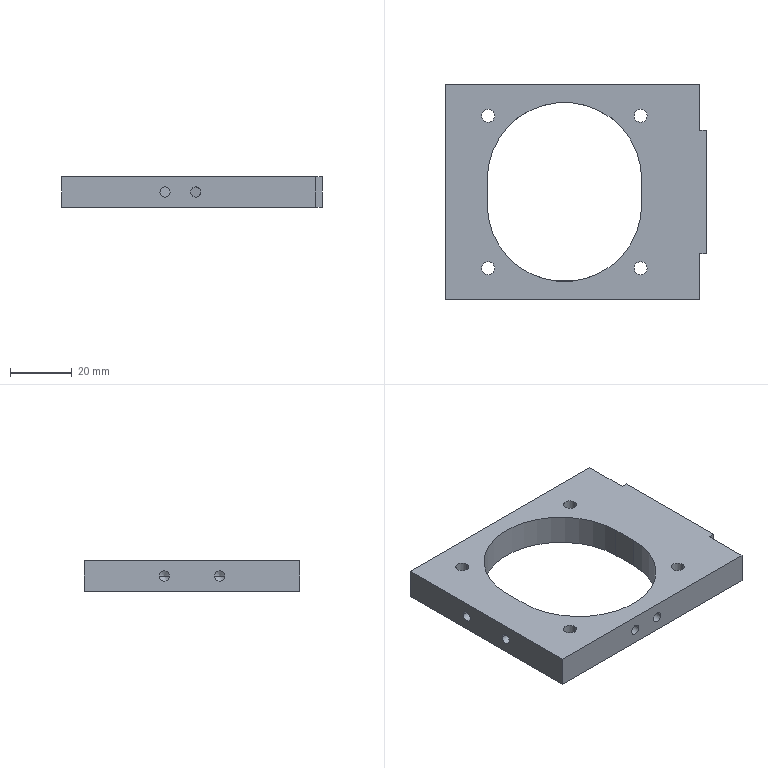Part | 1 solid | 42 faces | box 84.5 x 70 x 10 mm | volume 33501 mm3 | cylinder 22 | plane 12 | cone 8 | commonest cylinder face diameters 4.2 x12 3.3 x8 50.2 x2
STEP:
#1=CARTESIAN_POINT('',(-32.25,-7.35,-5.));
#2=VERTEX_POINT('',#1);
#3=CARTESIAN_POINT('',(-32.25,-10.65,-5.));
#4=VERTEX_POINT('',#3);
#5=CARTESIAN_POINT('',(-32.25,-9.,-5.));
#6=DIRECTION('',(-1.,0.,0.));
#7=DIRECTION('',(0.,-1.,0.));
#8=AXIS2_PLACEMENT_3D('',#5,#6,#7);
#9=CIRCLE('',#8,1.65);
#10=EDGE_CURVE('',#2,#4,#9,.T.);
#11=ORIENTED_EDGE('',*,*,#10,.F.);
#12=CARTESIAN_POINT('',(-42.25,-7.35,-5.));
#13=VERTEX_POINT('',#12);
#14=CARTESIAN_POINT('',(-42.25,-7.35,-5.));
#15=DIRECTION('',(-1.,0.,0.));
#16=VECTOR('',#15,1000.);
#17=LINE('',#14,#16);
#18=EDGE_CURVE('',#2,#13,#17,.T.);
#19=ORIENTED_EDGE('',*,*,#18,.T.);
#20=CARTESIAN_POINT('',(-42.25,-10.65,-5.));
#21=VERTEX_POINT('',#20);
#22=CARTESIAN_POINT('',(-42.25,-9.,-5.));
#23=DIRECTION('',(-1.,0.,0.));
#24=DIRECTION('',(0.,-1.,0.));
#25=AXIS2_PLACEMENT_3D('',#22,#23,#24);
#26=CIRCLE('',#25,1.65);
#27=EDGE_CURVE('',#13,#21,#26,.T.);
#28=ORIENTED_EDGE('',*,*,#27,.T.);
#29=CARTESIAN_POINT('',(-42.25,-10.65,-5.));
#30=DIRECTION('',(-1.,0.,0.));
#31=VECTOR('',#30,1000.);
#32=LINE('',#29,#31);
#33=EDGE_CURVE('',#4,#21,#32,.T.);
#34=ORIENTED_EDGE('',*,*,#33,.F.);
#35=EDGE_LOOP('',(#11,#19,#28,#34));
#36=FACE_BOUND('',#35,.T.);
#37=CARTESIAN_POINT('',(-42.25,-9.,-5.));
#38=DIRECTION('',(-1.,0.,0.));
#39=DIRECTION('',(0.,1.,0.));
#40=AXIS2_PLACEMENT_3D('',#37,#38,#39);
#41=CYLINDRICAL_SURFACE('',#40,1.65);
#42=ADVANCED_FACE('',(#36),#41,.F.);
#43=CARTESIAN_POINT('',(-31.259,-9.,-5.));
#44=VERTEX_POINT('',#43);
#45=CARTESIAN_POINT('',(-32.25,-10.65,-5.));
#46=DIRECTION('',(-0.515,-0.8572,0.));
#47=VECTOR('',#46,1000.);
#48=LINE('',#45,#47);
#49=EDGE_CURVE('',#44,#4,#48,.T.);
#50=ORIENTED_EDGE('',*,*,#49,.F.);
#51=CARTESIAN_POINT('',(-32.25,-7.35,-5.));
#52=DIRECTION('',(-0.515,0.8572,0.));
#53=VECTOR('',#52,1000.);
#54=LINE('',#51,#53);
#55=EDGE_CURVE('',#44,#2,#54,.T.);
#56=ORIENTED_EDGE('',*,*,#55,.T.);
#57=ORIENTED_EDGE('',*,*,#10,.T.);
#58=EDGE_LOOP('',(#50,#56,#57));
#59=FACE_BOUND('',#58,.T.);
#60=CARTESIAN_POINT('',(-32.25,-9.,-5.));
#61=DIRECTION('',(-1.,0.,0.));
#62=DIRECTION('',(0.,1.,0.));
#63=AXIS2_PLACEMENT_3D('',#60,#61,#62);
#64=CONICAL_SURFACE('',#63,1.65,1.03);
#65=ADVANCED_FACE('',(#59),#64,.F.);
#66=CARTESIAN_POINT('',(-32.25,10.65,-5.));
#67=VERTEX_POINT('',#66);
#68=CARTESIAN_POINT('',(-32.25,7.35,-5.));
#69=VERTEX_POINT('',#68);
#70=CARTESIAN_POINT('',(-32.25,9.,-5.));
#71=DIRECTION('',(-1.,0.,0.));
#72=DIRECTION('',(0.,-1.,0.));
#73=AXIS2_PLACEMENT_3D('',#70,#71,#72);
#74=CIRCLE('',#73,1.65);
#75=EDGE_CURVE('',#67,#69,#74,.T.);
#76=ORIENTED_EDGE('',*,*,#75,.F.);
#77=CARTESIAN_POINT('',(-42.25,10.65,-5.));
#78=VERTEX_POINT('',#77);
#79=CARTESIAN_POINT('',(-42.25,10.65,-5.));
#80=DIRECTION('',(-1.,0.,0.));
#81=VECTOR('',#80,1000.);
#82=LINE('',#79,#81);
#83=EDGE_CURVE('',#67,#78,#82,.T.);
#84=ORIENTED_EDGE('',*,*,#83,.T.);
#85=CARTESIAN_POINT('',(-42.25,7.35,-5.));
#86=VERTEX_POINT('',#85);
#87=CARTESIAN_POINT('',(-42.25,9.,-5.));
#88=DIRECTION('',(-1.,0.,0.));
#89=DIRECTION('',(0.,-1.,0.));
#90=AXIS2_PLACEMENT_3D('',#87,#88,#89);
#91=CIRCLE('',#90,1.65);
#92=EDGE_CURVE('',#78,#86,#91,.T.);
#93=ORIENTED_EDGE('',*,*,#92,.T.);
#94=CARTESIAN_POINT('',(-42.25,7.35,-5.));
#95=DIRECTION('',(-1.,0.,0.));
#96=VECTOR('',#95,1000.);
#97=LINE('',#94,#96);
#98=EDGE_CURVE('',#69,#86,#97,.T.);
#99=ORIENTED_EDGE('',*,*,#98,.F.);
#100=EDGE_LOOP('',(#76,#84,#93,#99));
#101=FACE_BOUND('',#100,.T.);
#102=CARTESIAN_POINT('',(-42.25,9.,-5.));
#103=DIRECTION('',(-1.,0.,0.));
#104=DIRECTION('',(0.,1.,0.));
#105=AXIS2_PLACEMENT_3D('',#102,#103,#104);
#106=CYLINDRICAL_SURFACE('',#105,1.65);
#107=ADVANCED_FACE('',(#101),#106,.F.);
#108=CARTESIAN_POINT('',(-31.259,9.,-5.));
#109=VERTEX_POINT('',#108);
#110=CARTESIAN_POINT('',(-32.25,7.35,-5.));
#111=DIRECTION('',(-0.515,-0.8572,0.));
#112=VECTOR('',#111,1000.);
#113=LINE('',#110,#112);
#114=EDGE_CURVE('',#109,#69,#113,.T.);
#115=ORIENTED_EDGE('',*,*,#114,.F.);
#116=CARTESIAN_POINT('',(-32.25,10.65,-5.));
#117=DIRECTION('',(-0.515,0.8572,0.));
#118=VECTOR('',#117,1000.);
#119=LINE('',#116,#118);
#120=EDGE_CURVE('',#109,#67,#119,.T.);
#121=ORIENTED_EDGE('',*,*,#120,.T.);
#122=ORIENTED_EDGE('',*,*,#75,.T.);
#123=EDGE_LOOP('',(#115,#121,#122));
#124=FACE_BOUND('',#123,.T.);
#125=CARTESIAN_POINT('',(-32.25,9.,-5.));
#126=DIRECTION('',(-1.,0.,0.));
#127=DIRECTION('',(0.,1.,0.));
#128=AXIS2_PLACEMENT_3D('',#125,#126,#127);
#129=CONICAL_SURFACE('',#128,1.65,1.03);
#130=ADVANCED_FACE('',(#124),#129,.F.);
#131=CARTESIAN_POINT('',(-10.4,-28.203,-5.));
#132=VERTEX_POINT('',#131);
#133=CARTESIAN_POINT('',(-7.1,-28.875,-5.));
#134=VERTEX_POINT('',#133);
#135=CARTESIAN_POINT('',(-10.4,-28.203,-5.));
#136=CARTESIAN_POINT('',(-10.4,-28.203,-5.441));
#137=CARTESIAN_POINT('',(-10.032,-28.308,-6.297));
#138=CARTESIAN_POINT('',(-8.762,-28.609,-6.824));
#139=CARTESIAN_POINT('',(-7.469,-28.83,-6.305));
#140=CARTESIAN_POINT('',(-7.1,-28.875,-5.441));
#141=CARTESIAN_POINT('',(-7.1,-28.875,-5.));
#142=B_SPLINE_CURVE_WITH_KNOTS('',3,(#135,#136,#137,#138,#139,#140,#141),.UNSPECIFIED.,.F.,.F.,(4,1,1,1,4),(0.,0.001303,0.002606,0.00391,0.005213),.UNSPECIFIED.);
#143=EDGE_CURVE('',#132,#134,#142,.T.);
#144=ORIENTED_EDGE('',*,*,#143,.F.);
#145=CARTESIAN_POINT('',(-10.4,-35.,-5.));
#146=VERTEX_POINT('',#145);
#147=CARTESIAN_POINT('',(-10.4,-35.,-5.));
#148=DIRECTION('',(0.,-1.,0.));
#149=VECTOR('',#148,1000.);
#150=LINE('',#147,#149);
#151=EDGE_CURVE('',#132,#146,#150,.T.);
#152=ORIENTED_EDGE('',*,*,#151,.T.);
#153=CARTESIAN_POINT('',(-7.1,-35.,-5.));
#154=VERTEX_POINT('',#153);
#155=CARTESIAN_POINT('',(-8.75,-35.,-5.));
#156=DIRECTION('',(0.,-1.,0.));
#157=DIRECTION('',(1.,0.,0.));
#158=AXIS2_PLACEMENT_3D('',#155,#156,#157);
#159=CIRCLE('',#158,1.65);
#160=EDGE_CURVE('',#146,#154,#159,.T.);
#161=ORIENTED_EDGE('',*,*,#160,.T.);
#162=CARTESIAN_POINT('',(-7.1,-35.,-5.));
#163=DIRECTION('',(0.,-1.,0.));
#164=VECTOR('',#163,1000.);
#165=LINE('',#162,#164);
#166=EDGE_CURVE('',#134,#154,#165,.T.);
#167=ORIENTED_EDGE('',*,*,#166,.F.);
#168=EDGE_LOOP('',(#144,#152,#161,#167));
#169=FACE_BOUND('',#168,.T.);
#170=CARTESIAN_POINT('',(-8.75,-35.,-5.));
#171=DIRECTION('',(0.,-1.,0.));
#172=DIRECTION('',(-1.,0.,0.));
#173=AXIS2_PLACEMENT_3D('',#170,#171,#172);
#174=CYLINDRICAL_SURFACE('',#173,1.65);
#175=ADVANCED_FACE('',(#169),#174,.F.);
#176=CARTESIAN_POINT('',(-0.4,-28.875,-5.));
#177=VERTEX_POINT('',#176);
#178=CARTESIAN_POINT('',(2.9,-28.203,-5.));
#179=VERTEX_POINT('',#178);
#180=CARTESIAN_POINT('',(-0.4,-28.875,-5.));
#181=CARTESIAN_POINT('',(-0.4,-28.875,-5.441));
#182=CARTESIAN_POINT('',(-0.03213,-28.83,-6.304));
#183=CARTESIAN_POINT('',(1.261,-28.609,-6.825));
#184=CARTESIAN_POINT('',(2.532,-28.308,-6.298));
#185=CARTESIAN_POINT('',(2.9,-28.203,-5.441));
#186=CARTESIAN_POINT('',(2.9,-28.203,-5.));
#187=B_SPLINE_CURVE_WITH_KNOTS('',3,(#180,#181,#182,#183,#184,#185,#186),.UNSPECIFIED.,.F.,.F.,(4,1,1,1,4),(0.,0.001303,0.002607,0.00391,0.005213),.UNSPECIFIED.);
#188=EDGE_CURVE('',#177,#179,#187,.T.);
#189=ORIENTED_EDGE('',*,*,#188,.F.);
#190=CARTESIAN_POINT('',(-0.4,-35.,-5.));
#191=VERTEX_POINT('',#190);
#192=CARTESIAN_POINT('',(-0.4,-35.,-5.));
#193=DIRECTION('',(0.,-1.,0.));
#194=VECTOR('',#193,1000.);
#195=LINE('',#192,#194);
#196=EDGE_CURVE('',#177,#191,#195,.T.);
#197=ORIENTED_EDGE('',*,*,#196,.T.);
#198=CARTESIAN_POINT('',(2.9,-35.,-5.));
#199=VERTEX_POINT('',#198);
#200=CARTESIAN_POINT('',(1.25,-35.,-5.));
#201=DIRECTION('',(0.,-1.,0.));
#202=DIRECTION('',(1.,0.,0.));
#203=AXIS2_PLACEMENT_3D('',#200,#201,#202);
#204=CIRCLE('',#203,1.65);
#205=EDGE_CURVE('',#191,#199,#204,.T.);
#206=ORIENTED_EDGE('',*,*,#205,.T.);
#207=CARTESIAN_POINT('',(2.9,-35.,-5.));
#208=DIRECTION('',(0.,-1.,0.));
#209=VECTOR('',#208,1000.);
#210=LINE('',#207,#209);
#211=EDGE_CURVE('',#179,#199,#210,.T.);
#212=ORIENTED_EDGE('',*,*,#211,.F.);
#213=EDGE_LOOP('',(#189,#197,#206,#212));
#214=FACE_BOUND('',#213,.T.);
#215=CARTESIAN_POINT('',(1.25,-35.,-5.));
#216=DIRECTION('',(0.,-1.,0.));
#217=DIRECTION('',(-1.,0.,0.));
#218=AXIS2_PLACEMENT_3D('',#215,#216,#217);
#219=CYLINDRICAL_SURFACE('',#218,1.65);
#220=ADVANCED_FACE('',(#214),#219,.F.);
#221=CARTESIAN_POINT('',(28.25,10.4,-5.));
#222=VERTEX_POINT('',#221);
#223=CARTESIAN_POINT('',(28.25,14.6,-5.));
#224=VERTEX_POINT('',#223);
#225=CARTESIAN_POINT('',(28.25,12.5,-5.));
#226=DIRECTION('',(1.,0.,0.));
#227=DIRECTION('',(0.,1.,0.));
#228=AXIS2_PLACEMENT_3D('',#225,#226,#227);
#229=CIRCLE('',#228,2.1);
#230=EDGE_CURVE('',#222,#224,#229,.T.);
#231=ORIENTED_EDGE('',*,*,#230,.F.);
#232=CARTESIAN_POINT('',(42.25,10.4,-5.));
#233=VERTEX_POINT('',#232);
#234=CARTESIAN_POINT('',(42.25,10.4,-5.));
#235=DIRECTION('',(1.,0.,0.));
#236=VECTOR('',#235,1000.);
#237=LINE('',#234,#236);
#238=EDGE_CURVE('',#222,#233,#237,.T.);
#239=ORIENTED_EDGE('',*,*,#238,.T.);
#240=CARTESIAN_POINT('',(42.25,14.6,-5.));
#241=VERTEX_POINT('',#240);
#242=CARTESIAN_POINT('',(42.25,12.5,-5.));
#243=DIRECTION('',(1.,0.,0.));
#244=DIRECTION('',(0.,1.,0.));
#245=AXIS2_PLACEMENT_3D('',#242,#243,#244);
#246=CIRCLE('',#245,2.1);
#247=EDGE_CURVE('',#233,#241,#246,.T.);
#248=ORIENTED_EDGE('',*,*,#247,.T.);
#249=CARTESIAN_POINT('',(42.25,14.6,-5.));
#250=DIRECTION('',(1.,0.,0.));
#251=VECTOR('',#250,1000.);
#252=LINE('',#249,#251);
#253=EDGE_CURVE('',#224,#241,#252,.T.);
#254=ORIENTED_EDGE('',*,*,#253,.F.);
#255=EDGE_LOOP('',(#231,#239,#248,#254));
#256=FACE_BOUND('',#255,.T.);
#257=CARTESIAN_POINT('',(42.25,12.5,-5.));
#258=DIRECTION('',(1.,0.,0.));
#259=DIRECTION('',(0.,-1.,0.));
#260=AXIS2_PLACEMENT_3D('',#257,#258,#259);
#261=CYLINDRICAL_SURFACE('',#260,2.1);
#262=ADVANCED_FACE('',(#256),#261,.F.);
#263=CARTESIAN_POINT('',(26.988,12.5,-5.));
#264=VERTEX_POINT('',#263);
#265=CARTESIAN_POINT('',(28.25,14.6,-5.));
#266=DIRECTION('',(0.515,0.8572,0.));
#267=VECTOR('',#266,1000.);
#268=LINE('',#265,#267);
#269=EDGE_CURVE('',#264,#224,#268,.T.);
#270=ORIENTED_EDGE('',*,*,#269,.F.);
#271=CARTESIAN_POINT('',(28.25,10.4,-5.));
#272=DIRECTION('',(0.515,-0.8572,0.));
#273=VECTOR('',#272,1000.);
#274=LINE('',#271,#273);
#275=EDGE_CURVE('',#264,#222,#274,.T.);
#276=ORIENTED_EDGE('',*,*,#275,.T.);
#277=ORIENTED_EDGE('',*,*,#230,.T.);
#278=EDGE_LOOP('',(#270,#276,#277));
#279=FACE_BOUND('',#278,.T.);
#280=CARTESIAN_POINT('',(28.25,12.5,-5.));
#281=DIRECTION('',(1.,0.,0.));
#282=DIRECTION('',(0.,-1.,0.));
#283=AXIS2_PLACEMENT_3D('',#280,#281,#282);
#284=CONICAL_SURFACE('',#283,2.1,1.03);
#285=ADVANCED_FACE('',(#279),#284,.F.);
#286=CARTESIAN_POINT('',(28.25,-14.6,-5.));
#287=VERTEX_POINT('',#286);
#288=CARTESIAN_POINT('',(28.25,-10.4,-5.));
#289=VERTEX_POINT('',#288);
#290=CARTESIAN_POINT('',(28.25,-12.5,-5.));
#291=DIRECTION('',(1.,0.,0.));
#292=DIRECTION('',(0.,1.,0.));
#293=AXIS2_PLACEMENT_3D('',#290,#291,#292);
#294=CIRCLE('',#293,2.1);
#295=EDGE_CURVE('',#287,#289,#294,.T.);
#296=ORIENTED_EDGE('',*,*,#295,.F.);
#297=CARTESIAN_POINT('',(42.25,-14.6,-5.));
#298=VERTEX_POINT('',#297);
#299=CARTESIAN_POINT('',(42.25,-14.6,-5.));
#300=DIRECTION('',(1.,0.,0.));
#301=VECTOR('',#300,1000.);
#302=LINE('',#299,#301);
#303=EDGE_CURVE('',#287,#298,#302,.T.);
#304=ORIENTED_EDGE('',*,*,#303,.T.);
#305=CARTESIAN_POINT('',(42.25,-10.4,-5.));
#306=VERTEX_POINT('',#305);
#307=CARTESIAN_POINT('',(42.25,-12.5,-5.));
#308=DIRECTION('',(1.,0.,0.));
#309=DIRECTION('',(0.,1.,0.));
#310=AXIS2_PLACEMENT_3D('',#307,#308,#309);
#311=CIRCLE('',#310,2.1);
#312=EDGE_CURVE('',#298,#306,#311,.T.);
#313=ORIENTED_EDGE('',*,*,#312,.T.);
#314=CARTESIAN_POINT('',(42.25,-10.4,-5.));
#315=DIRECTION('',(1.,0.,0.));
#316=VECTOR('',#315,1000.);
#317=LINE('',#314,#316);
#318=EDGE_CURVE('',#289,#306,#317,.T.);
#319=ORIENTED_EDGE('',*,*,#318,.F.);
#320=EDGE_LOOP('',(#296,#304,#313,#319));
#321=FACE_BOUND('',#320,.T.);
#322=CARTESIAN_POINT('',(42.25,-12.5,-5.));
#323=DIRECTION('',(1.,0.,0.));
#324=DIRECTION('',(0.,-1.,0.));
#325=AXIS2_PLACEMENT_3D('',#322,#323,#324);
#326=CYLINDRICAL_SURFACE('',#325,2.1);
#327=ADVANCED_FACE('',(#321),#326,.F.);
#328=CARTESIAN_POINT('',(26.988,-12.5,-5.));
#329=VERTEX_POINT('',#328);
#330=CARTESIAN_POINT('',(28.25,-10.4,-5.));
#331=DIRECTION('',(0.515,0.8572,0.));
#332=VECTOR('',#331,1000.);
#333=LINE('',#330,#332);
#334=EDGE_CURVE('',#329,#289,#333,.T.);
#335=ORIENTED_EDGE('',*,*,#334,.F.);
#336=CARTESIAN_POINT('',(28.25,-14.6,-5.));
#337=DIRECTION('',(0.515,-0.8572,0.));
#338=VECTOR('',#337,1000.);
#339=LINE('',#336,#338);
#340=EDGE_CURVE('',#329,#287,#339,.T.);
#341=ORIENTED_EDGE('',*,*,#340,.T.);
#342=ORIENTED_EDGE('',*,*,#295,.T.);
#343=EDGE_LOOP('',(#335,#341,#342));
#344=FACE_BOUND('',#343,.T.);
#345=CARTESIAN_POINT('',(28.25,-12.5,-5.));
#346=DIRECTION('',(1.,0.,0.));
#347=DIRECTION('',(0.,-1.,0.));
#348=AXIS2_PLACEMENT_3D('',#345,#346,#347);
#349=CONICAL_SURFACE('',#348,2.1,1.03);
#350=ADVANCED_FACE('',(#344),#349,.F.);
#351=CARTESIAN_POINT('',(-26.4,24.75,0.));
#352=VERTEX_POINT('',#351);
#353=CARTESIAN_POINT('',(-30.6,24.75,0.));
#354=VERTEX_POINT('',#353);
#355=CARTESIAN_POINT('',(-28.5,24.75,0.));
#356=DIRECTION('',(0.,0.,-1.));
#357=DIRECTION('',(-1.,0.,0.));
#358=AXIS2_PLACEMENT_3D('',#355,#356,#357);
#359=CIRCLE('',#358,2.1);
#360=EDGE_CURVE('',#352,#354,#359,.T.);
#361=ORIENTED_EDGE('',*,*,#360,.F.);
#362=CARTESIAN_POINT('',(-26.4,24.75,-10.));
#363=VERTEX_POINT('',#362);
#364=CARTESIAN_POINT('',(-26.4,24.75,-10.));
#365=DIRECTION('',(0.,0.,-1.));
#366=VECTOR('',#365,1000.);
#367=LINE('',#364,#366);
#368=EDGE_CURVE('',#352,#363,#367,.T.);
#369=ORIENTED_EDGE('',*,*,#368,.T.);
#370=CARTESIAN_POINT('',(-30.6,24.75,-10.));
#371=VERTEX_POINT('',#370);
#372=CARTESIAN_POINT('',(-28.5,24.75,-10.));
#373=DIRECTION('',(0.,0.,-1.));
#374=DIRECTION('',(-1.,0.,0.));
#375=AXIS2_PLACEMENT_3D('',#372,#373,#374);
#376=CIRCLE('',#375,2.1);
#377=EDGE_CURVE('',#363,#371,#376,.T.);
#378=ORIENTED_EDGE('',*,*,#377,.T.);
#379=CARTESIAN_POINT('',(-30.6,24.75,-10.));
#380=DIRECTION('',(0.,0.,-1.));
#381=VECTOR('',#380,1000.);
#382=LINE('',#379,#381);
#383=EDGE_CURVE('',#354,#371,#382,.T.);
#384=ORIENTED_EDGE('',*,*,#383,.F.);
#385=EDGE_LOOP('',(#361,#369,#378,#384));
#386=FACE_BOUND('',#385,.T.);
#387=CARTESIAN_POINT('',(-28.5,24.75,-10.));
#388=DIRECTION('',(0.,0.,-1.));
#389=DIRECTION('',(1.,0.,0.));
#390=AXIS2_PLACEMENT_3D('',#387,#388,#389);
#391=CYLINDRICAL_SURFACE('',#390,2.1);
#392=ADVANCED_FACE('',(#386),#391,.F.);
#393=CARTESIAN_POINT('',(-26.4,-24.75,0.));
#394=VERTEX_POINT('',#393);
#395=CARTESIAN_POINT('',(-30.6,-24.75,0.));
#396=VERTEX_POINT('',#395);
#397=CARTESIAN_POINT('',(-28.5,-24.75,0.));
#398=DIRECTION('',(0.,0.,-1.));
#399=DIRECTION('',(-1.,0.,0.));
#400=AXIS2_PLACEMENT_3D('',#397,#398,#399);
#401=CIRCLE('',#400,2.1);
#402=EDGE_CURVE('',#394,#396,#401,.T.);
#403=ORIENTED_EDGE('',*,*,#402,.F.);
#404=CARTESIAN_POINT('',(-26.4,-24.75,-10.));
#405=VERTEX_POINT('',#404);
#406=CARTESIAN_POINT('',(-26.4,-24.75,-10.));
#407=DIRECTION('',(0.,0.,-1.));
#408=VECTOR('',#407,1000.);
#409=LINE('',#406,#408);
#410=EDGE_CURVE('',#394,#405,#409,.T.);
#411=ORIENTED_EDGE('',*,*,#410,.T.);
#412=CARTESIAN_POINT('',(-30.6,-24.75,-10.));
#413=VERTEX_POINT('',#412);
#414=CARTESIAN_POINT('',(-28.5,-24.75,-10.));
#415=DIRECTION('',(0.,0.,-1.));
#416=DIRECTION('',(-1.,0.,0.));
#417=AXIS2_PLACEMENT_3D('',#414,#415,#416);
#418=CIRCLE('',#417,2.1);
#419=EDGE_CURVE('',#405,#413,#418,.T.);
#420=ORIENTED_EDGE('',*,*,#419,.T.);
#421=CARTESIAN_POINT('',(-30.6,-24.75,-10.));
#422=DIRECTION('',(0.,0.,-1.));
#423=VECTOR('',#422,1000.);
#424=LINE('',#421,#423);
#425=EDGE_CURVE('',#396,#413,#424,.T.);
#426=ORIENTED_EDGE('',*,*,#425,.F.);
#427=EDGE_LOOP('',(#403,#411,#420,#426));
#428=FACE_BOUND('',#427,.T.);
#429=CARTESIAN_POINT('',(-28.5,-24.75,-10.));
#430=DIRECTION('',(0.,0.,-1.));
#431=DIRECTION('',(1.,0.,0.));
#432=AXIS2_PLACEMENT_3D('',#429,#430,#431);
#433=CYLINDRICAL_SURFACE('',#432,2.1);
#434=ADVANCED_FACE('',(#428),#433,.F.);
#435=CARTESIAN_POINT('',(23.1,24.75,0.));
#436=VERTEX_POINT('',#435);
#437=CARTESIAN_POINT('',(18.9,24.75,0.));
#438=VERTEX_POINT('',#437);
#439=CARTESIAN_POINT('',(21.,24.75,0.));
#440=DIRECTION('',(0.,0.,-1.));
#441=DIRECTION('',(-1.,0.,0.));
#442=AXIS2_PLACEMENT_3D('',#439,#440,#441);
#443=CIRCLE('',#442,2.1);
#444=EDGE_CURVE('',#436,#438,#443,.T.);
#445=ORIENTED_EDGE('',*,*,#444,.F.);
#446=CARTESIAN_POINT('',(23.1,24.75,-10.));
#447=VERTEX_POINT('',#446);
#448=CARTESIAN_POINT('',(23.1,24.75,-10.));
#449=DIRECTION('',(0.,0.,-1.));
#450=VECTOR('',#449,1000.);
#451=LINE('',#448,#450);
#452=EDGE_CURVE('',#436,#447,#451,.T.);
#453=ORIENTED_EDGE('',*,*,#452,.T.);
#454=CARTESIAN_POINT('',(18.9,24.75,-10.));
#455=VERTEX_POINT('',#454);
#456=CARTESIAN_POINT('',(21.,24.75,-10.));
#457=DIRECTION('',(0.,0.,-1.));
#458=DIRECTION('',(-1.,0.,0.));
#459=AXIS2_PLACEMENT_3D('',#456,#457,#458);
#460=CIRCLE('',#459,2.1);
#461=EDGE_CURVE('',#447,#455,#460,.T.);
#462=ORIENTED_EDGE('',*,*,#461,.T.);
#463=CARTESIAN_POINT('',(18.9,24.75,-10.));
#464=DIRECTION('',(0.,0.,-1.));
#465=VECTOR('',#464,1000.);
#466=LINE('',#463,#465);
#467=EDGE_CURVE('',#438,#455,#466,.T.);
#468=ORIENTED_EDGE('',*,*,#467,.F.);
#469=EDGE_LOOP('',(#445,#453,#462,#468));
#470=FACE_BOUND('',#469,.T.);
#471=CARTESIAN_POINT('',(21.,24.75,-10.));
#472=DIRECTION('',(0.,0.,-1.));
#473=DIRECTION('',(1.,0.,0.));
#474=AXIS2_PLACEMENT_3D('',#471,#472,#473);
#475=CYLINDRICAL_SURFACE('',#474,2.1);
#476=ADVANCED_FACE('',(#470),#475,.F.);
#477=CARTESIAN_POINT('',(23.1,-24.75,0.));
#478=VERTEX_POINT('',#477);
#479=CARTESIAN_POINT('',(18.9,-24.75,0.));
#480=VERTEX_POINT('',#479);
#481=CARTESIAN_POINT('',(21.,-24.75,0.));
#482=DIRECTION('',(0.,0.,-1.));
#483=DIRECTION('',(-1.,0.,0.));
#484=AXIS2_PLACEMENT_3D('',#481,#482,#483);
#485=CIRCLE('',#484,2.1);
#486=EDGE_CURVE('',#478,#480,#485,.T.);
#487=ORIENTED_EDGE('',*,*,#486,.F.);
#488=CARTESIAN_POINT('',(23.1,-24.75,-10.));
#489=VERTEX_POINT('',#488);
#490=CARTESIAN_POINT('',(23.1,-24.75,-10.));
#491=DIRECTION('',(0.,0.,-1.));
#492=VECTOR('',#491,1000.);
#493=LINE('',#490,#492);
#494=EDGE_CURVE('',#478,#489,#493,.T.);
#495=ORIENTED_EDGE('',*,*,#494,.T.);
#496=CARTESIAN_POINT('',(18.9,-24.75,-10.));
#497=VERTEX_POINT('',#496);
#498=CARTESIAN_POINT('',(21.,-24.75,-10.));
#499=DIRECTION('',(0.,0.,-1.));
#500=DIRECTION('',(-1.,0.,0.));
#501=AXIS2_PLACEMENT_3D('',#498,#499,#500);
#502=CIRCLE('',#501,2.1);
#503=EDGE_CURVE('',#489,#497,#502,.T.);
#504=ORIENTED_EDGE('',*,*,#503,.T.);
#505=CARTESIAN_POINT('',(18.9,-24.75,-10.));
#506=DIRECTION('',(0.,0.,-1.));
#507=VECTOR('',#506,1000.);
#508=LINE('',#505,#507);
#509=EDGE_CURVE('',#480,#497,#508,.T.);
#510=ORIENTED_EDGE('',*,*,#509,.F.);
#511=EDGE_LOOP('',(#487,#495,#504,#510));
#512=FACE_BOUND('',#511,.T.);
#513=CARTESIAN_POINT('',(21.,-24.75,-10.));
#514=DIRECTION('',(0.,0.,-1.));
#515=DIRECTION('',(1.,0.,0.));
#516=AXIS2_PLACEMENT_3D('',#513,#514,#515);
#517=CYLINDRICAL_SURFACE('',#516,2.1);
#518=ADVANCED_FACE('',(#512),#517,.F.);
#519=CARTESIAN_POINT('',(40.25,35.,0.));
#520=VERTEX_POINT('',#519);
#521=CARTESIAN_POINT('',(-42.25,35.,0.));
#522=VERTEX_POINT('',#521);
#523=CARTESIAN_POINT('',(42.25,35.,0.));
#524=DIRECTION('',(-1.,0.,0.));
#525=VECTOR('',#524,1000.);
#526=LINE('',#523,#525);
#527=EDGE_CURVE('',#520,#522,#526,.T.);
#528=ORIENTED_EDGE('',*,*,#527,.F.);
#529=CARTESIAN_POINT('',(40.25,35.,-10.));
#530=VERTEX_POINT('',#529);
#531=CARTESIAN_POINT('',(40.25,35.,0.));
#532=DIRECTION('',(0.,0.,-1.));
#533=VECTOR('',#532,1000.);
#534=LINE('',#531,#533);
#535=EDGE_CURVE('',#520,#530,#534,.T.);
#536=ORIENTED_EDGE('',*,*,#535,.T.);
#537=CARTESIAN_POINT('',(-42.25,35.,-10.));
#538=VERTEX_POINT('',#537);
#539=CARTESIAN_POINT('',(42.25,35.,-10.));
#540=DIRECTION('',(-1.,0.,0.));
#541=VECTOR('',#540,1000.);
#542=LINE('',#539,#541);
#543=EDGE_CURVE('',#530,#538,#542,.T.);
#544=ORIENTED_EDGE('',*,*,#543,.T.);
#545=CARTESIAN_POINT('',(-42.25,35.,0.));
#546=DIRECTION('',(0.,0.,-1.));
#547=VECTOR('',#546,1000.);
#548=LINE('',#545,#547);
#549=EDGE_CURVE('',#522,#538,#548,.T.);
#550=ORIENTED_EDGE('',*,*,#549,.F.);
#551=EDGE_LOOP('',(#528,#536,#544,#550));
#552=FACE_BOUND('',#551,.T.);
#553=CARTESIAN_POINT('',(42.25,35.,0.));
#554=DIRECTION('',(0.,-1.,0.));
#555=DIRECTION('',(-1.,0.,0.));
#556=AXIS2_PLACEMENT_3D('',#553,#554,#555);
#557=PLANE('',#556);
#558=ADVANCED_FACE('',(#552),#557,.F.);
#559=CARTESIAN_POINT('',(-42.25,-9.,-5.));
#560=DIRECTION('',(-1.,0.,0.));
#561=DIRECTION('',(0.,-1.,0.));
#562=AXIS2_PLACEMENT_3D('',#559,#560,#561);
#563=CIRCLE('',#562,1.65);
#564=EDGE_CURVE('',#21,#13,#563,.T.);
#565=ORIENTED_EDGE('',*,*,#564,.F.);
#566=ORIENTED_EDGE('',*,*,#27,.F.);
#567=EDGE_LOOP('',(#565,#566));
#568=FACE_BOUND('',#567,.T.);
#569=CARTESIAN_POINT('',(-42.25,9.,-5.));
#570=DIRECTION('',(-1.,0.,0.));
#571=DIRECTION('',(0.,-1.,0.));
#572=AXIS2_PLACEMENT_3D('',#569,#570,#571);
#573=CIRCLE('',#572,1.65);
#574=EDGE_CURVE('',#86,#78,#573,.T.);
#575=ORIENTED_EDGE('',*,*,#574,.F.);
#576=ORIENTED_EDGE('',*,*,#92,.F.);
#577=EDGE_LOOP('',(#575,#576));
#578=FACE_BOUND('',#577,.T.);
#579=CARTESIAN_POINT('',(-42.25,-35.,-10.));
#580=VERTEX_POINT('',#579);
#581=CARTESIAN_POINT('',(-42.25,-35.,-10.));
#582=DIRECTION('',(0.,-1.,0.));
#583=VECTOR('',#582,1000.);
#584=LINE('',#581,#583);
#585=EDGE_CURVE('',#538,#580,#584,.T.);
#586=ORIENTED_EDGE('',*,*,#585,.T.);
#587=CARTESIAN_POINT('',(-42.25,-35.,0.));
#588=VERTEX_POINT('',#587);
#589=CARTESIAN_POINT('',(-42.25,-35.,0.));
#590=DIRECTION('',(0.,0.,-1.));
#591=VECTOR('',#590,1000.);
#592=LINE('',#589,#591);
#593=EDGE_CURVE('',#588,#580,#592,.T.);
#594=ORIENTED_EDGE('',*,*,#593,.F.);
#595=CARTESIAN_POINT('',(-42.25,-35.,0.));
#596=DIRECTION('',(0.,-1.,0.));
#597=VECTOR('',#596,1000.);
#598=LINE('',#595,#597);
#599=EDGE_CURVE('',#522,#588,#598,.T.);
#600=ORIENTED_EDGE('',*,*,#599,.F.);
#601=ORIENTED_EDGE('',*,*,#549,.T.);
#602=EDGE_LOOP('',(#586,#594,#600,#601));
#603=FACE_BOUND('',#602,.T.);
#604=CARTESIAN_POINT('',(-42.25,-35.,0.));
#605=DIRECTION('',(1.,0.,0.));
#606=DIRECTION('',(0.,-1.,0.));
#607=AXIS2_PLACEMENT_3D('',#604,#605,#606);
#608=PLANE('',#607);
#609=ADVANCED_FACE('',(#568,#578,#603),#608,.F.);
#610=CARTESIAN_POINT('',(-8.75,-35.,-5.));
#611=DIRECTION('',(0.,-1.,0.));
#612=DIRECTION('',(1.,0.,0.));
#613=AXIS2_PLACEMENT_3D('',#610,#611,#612);
#614=CIRCLE('',#613,1.65);
#615=EDGE_CURVE('',#154,#146,#614,.T.);
#616=ORIENTED_EDGE('',*,*,#615,.F.);
#617=ORIENTED_EDGE('',*,*,#160,.F.);
#618=EDGE_LOOP('',(#616,#617));
#619=FACE_BOUND('',#618,.T.);
#620=CARTESIAN_POINT('',(1.25,-35.,-5.));
#621=DIRECTION('',(0.,-1.,0.));
#622=DIRECTION('',(1.,0.,0.));
#623=AXIS2_PLACEMENT_3D('',#620,#621,#622);
#624=CIRCLE('',#623,1.65);
#625=EDGE_CURVE('',#199,#191,#624,.T.);
#626=ORIENTED_EDGE('',*,*,#625,.F.);
#627=ORIENTED_EDGE('',*,*,#205,.F.);
#628=EDGE_LOOP('',(#626,#627));
#629=FACE_BOUND('',#628,.T.);
#630=CARTESIAN_POINT('',(40.25,-35.,-10.));
#631=VERTEX_POINT('',#630);
#632=CARTESIAN_POINT('',(42.25,-35.,-10.));
#633=DIRECTION('',(1.,0.,0.));
#634=VECTOR('',#633,1000.);
#635=LINE('',#632,#634);
#636=EDGE_CURVE('',#580,#631,#635,.T.);
#637=ORIENTED_EDGE('',*,*,#636,.T.);
#638=CARTESIAN_POINT('',(40.25,-35.,0.));
#639=VERTEX_POINT('',#638);
#640=CARTESIAN_POINT('',(40.25,-35.,0.));
#641=DIRECTION('',(0.,0.,-1.));
#642=VECTOR('',#641,1000.);
#643=LINE('',#640,#642);
#644=EDGE_CURVE('',#639,#631,#643,.T.);
#645=ORIENTED_EDGE('',*,*,#644,.F.);
#646=CARTESIAN_POINT('',(42.25,-35.,0.));
#647=DIRECTION('',(1.,0.,0.));
#648=VECTOR('',#647,1000.);
#649=LINE('',#646,#648);
#650=EDGE_CURVE('',#588,#639,#649,.T.);
#651=ORIENTED_EDGE('',*,*,#650,.F.);
#652=ORIENTED_EDGE('',*,*,#593,.T.);
#653=EDGE_LOOP('',(#637,#645,#651,#652));
#654=FACE_BOUND('',#653,.T.);
#655=CARTESIAN_POINT('',(42.25,-35.,0.));
#656=DIRECTION('',(0.,1.,0.));
#657=DIRECTION('',(1.,0.,0.));
#658=AXIS2_PLACEMENT_3D('',#655,#656,#657);
#659=PLANE('',#658);
#660=ADVANCED_FACE('',(#619,#629,#654),#659,.F.);
#661=CARTESIAN_POINT('',(42.25,12.5,-5.));
#662=DIRECTION('',(1.,0.,0.));
#663=DIRECTION('',(0.,1.,0.));
#664=AXIS2_PLACEMENT_3D('',#661,#662,#663);
#665=CIRCLE('',#664,2.1);
#666=EDGE_CURVE('',#241,#233,#665,.T.);
#667=ORIENTED_EDGE('',*,*,#666,.F.);
#668=ORIENTED_EDGE('',*,*,#247,.F.);
#669=EDGE_LOOP('',(#667,#668));
#670=FACE_BOUND('',#669,.T.);
#671=CARTESIAN_POINT('',(42.25,-12.5,-5.));
#672=DIRECTION('',(1.,0.,0.));
#673=DIRECTION('',(0.,1.,0.));
#674=AXIS2_PLACEMENT_3D('',#671,#672,#673);
#675=CIRCLE('',#674,2.1);
#676=EDGE_CURVE('',#306,#298,#675,.T.);
#677=ORIENTED_EDGE('',*,*,#676,.F.);
#678=ORIENTED_EDGE('',*,*,#312,.F.);
#679=EDGE_LOOP('',(#677,#678));
#680=FACE_BOUND('',#679,.T.);
#681=CARTESIAN_POINT('',(42.25,-20.,0.));
#682=VERTEX_POINT('',#681);
#683=CARTESIAN_POINT('',(42.25,20.,0.));
#684=VERTEX_POINT('',#683);
#685=CARTESIAN_POINT('',(42.25,-35.,0.));
#686=DIRECTION('',(0.,1.,0.));
#687=VECTOR('',#686,1000.);
#688=LINE('',#685,#687);
#689=EDGE_CURVE('',#682,#684,#688,.T.);
#690=ORIENTED_EDGE('',*,*,#689,.F.);
#691=CARTESIAN_POINT('',(42.25,-20.,-10.));
#692=VERTEX_POINT('',#691);
#693=CARTESIAN_POINT('',(42.25,-20.,0.));
#694=DIRECTION('',(0.,0.,-1.));
#695=VECTOR('',#694,1000.);
#696=LINE('',#693,#695);
#697=EDGE_CURVE('',#682,#692,#696,.T.);
#698=ORIENTED_EDGE('',*,*,#697,.T.);
#699=CARTESIAN_POINT('',(42.25,20.,-10.));
#700=VERTEX_POINT('',#699);
#701=CARTESIAN_POINT('',(42.25,-35.,-10.));
#702=DIRECTION('',(0.,1.,0.));
#703=VECTOR('',#702,1000.);
#704=LINE('',#701,#703);
#705=EDGE_CURVE('',#692,#700,#704,.T.);
#706=ORIENTED_EDGE('',*,*,#705,.T.);
#707=CARTESIAN_POINT('',(42.25,20.,0.));
#708=DIRECTION('',(0.,0.,-1.));
#709=VECTOR('',#708,1000.);
#710=LINE('',#707,#709);
#711=EDGE_CURVE('',#684,#700,#710,.T.);
#712=ORIENTED_EDGE('',*,*,#711,.F.);
#713=EDGE_LOOP('',(#690,#698,#706,#712));
#714=FACE_BOUND('',#713,.T.);
#715=CARTESIAN_POINT('',(42.25,-35.,0.));
#716=DIRECTION('',(-1.,0.,0.));
#717=DIRECTION('',(0.,1.,0.));
#718=AXIS2_PLACEMENT_3D('',#715,#716,#717);
#719=PLANE('',#718);
#720=ADVANCED_FACE('',(#670,#680,#714),#719,.F.);
#721=CARTESIAN_POINT('',(-28.5,24.75,0.));
#722=DIRECTION('',(0.,0.,-1.));
#723=DIRECTION('',(-1.,0.,0.));
#724=AXIS2_PLACEMENT_3D('',#721,#722,#723);
#725=CIRCLE('',#724,2.1);
#726=EDGE_CURVE('',#354,#352,#725,.T.);
#727=ORIENTED_EDGE('',*,*,#726,.T.);
#728=ORIENTED_EDGE('',*,*,#360,.T.);
#729=EDGE_LOOP('',(#727,#728));
#730=FACE_BOUND('',#729,.T.);
#731=CARTESIAN_POINT('',(-28.5,-24.75,0.));
#732=DIRECTION('',(0.,0.,-1.));
#733=DIRECTION('',(-1.,0.,0.));
#734=AXIS2_PLACEMENT_3D('',#731,#732,#733);
#735=CIRCLE('',#734,2.1);
#736=EDGE_CURVE('',#396,#394,#735,.T.);
#737=ORIENTED_EDGE('',*,*,#736,.T.);
#738=ORIENTED_EDGE('',*,*,#402,.T.);
#739=EDGE_LOOP('',(#737,#738));
#740=FACE_BOUND('',#739,.T.);
#741=CARTESIAN_POINT('',(21.,24.75,0.));
#742=DIRECTION('',(0.,0.,-1.));
#743=DIRECTION('',(-1.,0.,0.));
#744=AXIS2_PLACEMENT_3D('',#741,#742,#743);
#745=CIRCLE('',#744,2.1);
#746=EDGE_CURVE('',#438,#436,#745,.T.);
#747=ORIENTED_EDGE('',*,*,#746,.T.);
#748=ORIENTED_EDGE('',*,*,#444,.T.);
#749=EDGE_LOOP('',(#747,#748));
#750=FACE_BOUND('',#749,.T.);
#751=CARTESIAN_POINT('',(21.,-24.75,0.));
#752=DIRECTION('',(0.,0.,-1.));
#753=DIRECTION('',(-1.,0.,0.));
#754=AXIS2_PLACEMENT_3D('',#751,#752,#753);
#755=CIRCLE('',#754,2.1);
#756=EDGE_CURVE('',#480,#478,#755,.T.);
#757=ORIENTED_EDGE('',*,*,#756,.T.);
#758=ORIENTED_EDGE('',*,*,#486,.T.);
#759=EDGE_LOOP('',(#757,#758));
#760=FACE_BOUND('',#759,.T.);
#761=CARTESIAN_POINT('',(21.35,-4.,0.));
#762=VERTEX_POINT('',#761);
#763=CARTESIAN_POINT('',(21.35,4.,0.));
#764=VERTEX_POINT('',#763);
#765=CARTESIAN_POINT('',(21.35,-4.,0.));
#766=DIRECTION('',(0.,1.,0.));
#767=VECTOR('',#766,1000.);
#768=LINE('',#765,#767);
#769=EDGE_CURVE('',#762,#764,#768,.T.);
#770=ORIENTED_EDGE('',*,*,#769,.F.);
#771=CARTESIAN_POINT('',(-28.85,-4.,0.));
#772=VERTEX_POINT('',#771);
#773=CARTESIAN_POINT('',(-3.75,-4.,0.));
#774=DIRECTION('',(0.,0.,1.));
#775=DIRECTION('',(1.,0.,0.));
#776=AXIS2_PLACEMENT_3D('',#773,#774,#775);
#777=CIRCLE('',#776,25.1);
#778=EDGE_CURVE('',#772,#762,#777,.T.);
#779=ORIENTED_EDGE('',*,*,#778,.F.);
#780=CARTESIAN_POINT('',(-28.85,4.,0.));
#781=VERTEX_POINT('',#780);
#782=CARTESIAN_POINT('',(-28.85,-4.,0.));
#783=DIRECTION('',(0.,-1.,0.));
#784=VECTOR('',#783,1000.);
#785=LINE('',#782,#784);
#786=EDGE_CURVE('',#781,#772,#785,.T.);
#787=ORIENTED_EDGE('',*,*,#786,.F.);
#788=CARTESIAN_POINT('',(-3.75,4.,0.));
#789=DIRECTION('',(0.,0.,1.));
#790=DIRECTION('',(1.,0.,0.));
#791=AXIS2_PLACEMENT_3D('',#788,#789,#790);
#792=CIRCLE('',#791,25.1);
#793=EDGE_CURVE('',#764,#781,#792,.T.);
#794=ORIENTED_EDGE('',*,*,#793,.F.);
#795=EDGE_LOOP('',(#770,#779,#787,#794));
#796=FACE_BOUND('',#795,.T.);
#797=CARTESIAN_POINT('',(40.25,-20.,0.));
#798=VERTEX_POINT('',#797);
#799=CARTESIAN_POINT('',(40.25,-35.,0.));
#800=DIRECTION('',(0.,1.,0.));
#801=VECTOR('',#800,1000.);
#802=LINE('',#799,#801);
#803=EDGE_CURVE('',#639,#798,#802,.T.);
#804=ORIENTED_EDGE('',*,*,#803,.T.);
#805=CARTESIAN_POINT('',(42.25,-20.,0.));
#806=DIRECTION('',(1.,0.,0.));
#807=VECTOR('',#806,1000.);
#808=LINE('',#805,#807);
#809=EDGE_CURVE('',#798,#682,#808,.T.);
#810=ORIENTED_EDGE('',*,*,#809,.T.);
#811=ORIENTED_EDGE('',*,*,#689,.T.);
#812=CARTESIAN_POINT('',(40.25,20.,0.));
#813=VERTEX_POINT('',#812);
#814=CARTESIAN_POINT('',(42.25,20.,0.));
#815=DIRECTION('',(-1.,0.,0.));
#816=VECTOR('',#815,1000.);
#817=LINE('',#814,#816);
#818=EDGE_CURVE('',#684,#813,#817,.T.);
#819=ORIENTED_EDGE('',*,*,#818,.T.);
#820=CARTESIAN_POINT('',(40.25,35.,0.));
#821=DIRECTION('',(0.,1.,0.));
#822=VECTOR('',#821,1000.);
#823=LINE('',#820,#822);
#824=EDGE_CURVE('',#813,#520,#823,.T.);
#825=ORIENTED_EDGE('',*,*,#824,.T.);
#826=ORIENTED_EDGE('',*,*,#527,.T.);
#827=ORIENTED_EDGE('',*,*,#599,.T.);
#828=ORIENTED_EDGE('',*,*,#650,.T.);
#829=EDGE_LOOP('',(#804,#810,#811,#819,#825,#826,#827,#828));
#830=FACE_BOUND('',#829,.T.);
#831=CARTESIAN_POINT('',(0.,0.,0.));
#832=DIRECTION('',(0.,0.,-1.));
#833=DIRECTION('',(1.,0.,0.));
#834=AXIS2_PLACEMENT_3D('',#831,#832,#833);
#835=PLANE('',#834);
#836=ADVANCED_FACE('',(#730,#740,#750,#760,#796,#830),#835,.F.);
#837=CARTESIAN_POINT('',(-28.5,24.75,-10.));
#838=DIRECTION('',(0.,0.,-1.));
#839=DIRECTION('',(-1.,0.,0.));
#840=AXIS2_PLACEMENT_3D('',#837,#838,#839);
#841=CIRCLE('',#840,2.1);
#842=EDGE_CURVE('',#371,#363,#841,.T.);
#843=ORIENTED_EDGE('',*,*,#842,.F.);
#844=ORIENTED_EDGE('',*,*,#377,.F.);
#845=EDGE_LOOP('',(#843,#844));
#846=FACE_BOUND('',#845,.T.);
#847=CARTESIAN_POINT('',(-28.5,-24.75,-10.));
#848=DIRECTION('',(0.,0.,-1.));
#849=DIRECTION('',(-1.,0.,0.));
#850=AXIS2_PLACEMENT_3D('',#847,#848,#849);
#851=CIRCLE('',#850,2.1);
#852=EDGE_CURVE('',#413,#405,#851,.T.);
#853=ORIENTED_EDGE('',*,*,#852,.F.);
#854=ORIENTED_EDGE('',*,*,#419,.F.);
#855=EDGE_LOOP('',(#853,#854));
#856=FACE_BOUND('',#855,.T.);
#857=CARTESIAN_POINT('',(21.,24.75,-10.));
#858=DIRECTION('',(0.,0.,-1.));
#859=DIRECTION('',(-1.,0.,0.));
#860=AXIS2_PLACEMENT_3D('',#857,#858,#859);
#861=CIRCLE('',#860,2.1);
#862=EDGE_CURVE('',#455,#447,#861,.T.);
#863=ORIENTED_EDGE('',*,*,#862,.F.);
#864=ORIENTED_EDGE('',*,*,#461,.F.);
#865=EDGE_LOOP('',(#863,#864));
#866=FACE_BOUND('',#865,.T.);
#867=CARTESIAN_POINT('',(21.,-24.75,-10.));
#868=DIRECTION('',(0.,0.,-1.));
#869=DIRECTION('',(-1.,0.,0.));
#870=AXIS2_PLACEMENT_3D('',#867,#868,#869);
#871=CIRCLE('',#870,2.1);
#872=EDGE_CURVE('',#497,#489,#871,.T.);
#873=ORIENTED_EDGE('',*,*,#872,.F.);
#874=ORIENTED_EDGE('',*,*,#503,.F.);
#875=EDGE_LOOP('',(#873,#874));
#876=FACE_BOUND('',#875,.T.);
#877=CARTESIAN_POINT('',(40.25,-20.,-10.));
#878=VERTEX_POINT('',#877);
#879=CARTESIAN_POINT('',(42.25,-20.,-10.));
#880=DIRECTION('',(1.,0.,0.));
#881=VECTOR('',#880,1000.);
#882=LINE('',#879,#881);
#883=EDGE_CURVE('',#878,#692,#882,.T.);
#884=ORIENTED_EDGE('',*,*,#883,.F.);
#885=CARTESIAN_POINT('',(40.25,-35.,-10.));
#886=DIRECTION('',(0.,1.,0.));
#887=VECTOR('',#886,1000.);
#888=LINE('',#885,#887);
#889=EDGE_CURVE('',#631,#878,#888,.T.);
#890=ORIENTED_EDGE('',*,*,#889,.F.);
#891=ORIENTED_EDGE('',*,*,#636,.F.);
#892=ORIENTED_EDGE('',*,*,#585,.F.);
#893=ORIENTED_EDGE('',*,*,#543,.F.);
#894=CARTESIAN_POINT('',(40.25,20.,-10.));
#895=VERTEX_POINT('',#894);
#896=CARTESIAN_POINT('',(40.25,35.,-10.));
#897=DIRECTION('',(0.,1.,0.));
#898=VECTOR('',#897,1000.);
#899=LINE('',#896,#898);
#900=EDGE_CURVE('',#895,#530,#899,.T.);
#901=ORIENTED_EDGE('',*,*,#900,.F.);
#902=CARTESIAN_POINT('',(42.25,20.,-10.));
#903=DIRECTION('',(-1.,0.,0.));
#904=VECTOR('',#903,1000.);
#905=LINE('',#902,#904);
#906=EDGE_CURVE('',#700,#895,#905,.T.);
#907=ORIENTED_EDGE('',*,*,#906,.F.);
#908=ORIENTED_EDGE('',*,*,#705,.F.);
#909=EDGE_LOOP('',(#884,#890,#891,#892,#893,#901,#907,#908));
#910=FACE_BOUND('',#909,.T.);
#911=CARTESIAN_POINT('',(-28.85,-4.,-10.));
#912=VERTEX_POINT('',#911);
#913=CARTESIAN_POINT('',(21.35,-4.,-10.));
#914=VERTEX_POINT('',#913);
#915=CARTESIAN_POINT('',(-3.75,-4.,-10.));
#916=DIRECTION('',(0.,0.,1.));
#917=DIRECTION('',(1.,0.,0.));
#918=AXIS2_PLACEMENT_3D('',#915,#916,#917);
#919=CIRCLE('',#918,25.1);
#920=EDGE_CURVE('',#912,#914,#919,.T.);
#921=ORIENTED_EDGE('',*,*,#920,.T.);
#922=CARTESIAN_POINT('',(21.35,4.,-10.));
#923=VERTEX_POINT('',#922);
#924=CARTESIAN_POINT('',(21.35,-4.,-10.));
#925=DIRECTION('',(0.,1.,0.));
#926=VECTOR('',#925,1000.);
#927=LINE('',#924,#926);
#928=EDGE_CURVE('',#914,#923,#927,.T.);
#929=ORIENTED_EDGE('',*,*,#928,.T.);
#930=CARTESIAN_POINT('',(-28.85,4.,-10.));
#931=VERTEX_POINT('',#930);
#932=CARTESIAN_POINT('',(-3.75,4.,-10.));
#933=DIRECTION('',(0.,0.,1.));
#934=DIRECTION('',(1.,0.,0.));
#935=AXIS2_PLACEMENT_3D('',#932,#933,#934);
#936=CIRCLE('',#935,25.1);
#937=EDGE_CURVE('',#923,#931,#936,.T.);
#938=ORIENTED_EDGE('',*,*,#937,.T.);
#939=CARTESIAN_POINT('',(-28.85,-4.,-10.));
#940=DIRECTION('',(0.,-1.,0.));
#941=VECTOR('',#940,1000.);
#942=LINE('',#939,#941);
#943=EDGE_CURVE('',#931,#912,#942,.T.);
#944=ORIENTED_EDGE('',*,*,#943,.T.);
#945=EDGE_LOOP('',(#921,#929,#938,#944));
#946=FACE_BOUND('',#945,.T.);
#947=CARTESIAN_POINT('',(0.,0.,-10.));
#948=DIRECTION('',(0.,0.,-1.));
#949=DIRECTION('',(1.,0.,0.));
#950=AXIS2_PLACEMENT_3D('',#947,#948,#949);
#951=PLANE('',#950);
#952=ADVANCED_FACE('',(#846,#856,#866,#876,#910,#946),#951,.T.);
#953=ORIENTED_EDGE('',*,*,#943,.F.);
#954=CARTESIAN_POINT('',(-28.85,4.,-10.));
#955=DIRECTION('',(0.,0.,1.));
#956=VECTOR('',#955,1000.);
#957=LINE('',#954,#956);
#958=EDGE_CURVE('',#931,#781,#957,.T.);
#959=ORIENTED_EDGE('',*,*,#958,.T.);
#960=ORIENTED_EDGE('',*,*,#786,.T.);
#961=CARTESIAN_POINT('',(-28.85,-4.,-10.));
#962=DIRECTION('',(0.,0.,1.));
#963=VECTOR('',#962,1000.);
#964=LINE('',#961,#963);
#965=EDGE_CURVE('',#912,#772,#964,.T.);
#966=ORIENTED_EDGE('',*,*,#965,.F.);
#967=EDGE_LOOP('',(#953,#959,#960,#966));
#968=FACE_BOUND('',#967,.T.);
#969=CARTESIAN_POINT('',(-28.85,-4.,-10.));
#970=DIRECTION('',(-1.,0.,0.));
#971=DIRECTION('',(0.,1.,0.));
#972=AXIS2_PLACEMENT_3D('',#969,#970,#971);
#973=PLANE('',#972);
#974=ADVANCED_FACE('',(#968),#973,.F.);
#975=ORIENTED_EDGE('',*,*,#928,.F.);
#976=CARTESIAN_POINT('',(21.35,-4.,-10.));
#977=DIRECTION('',(0.,0.,1.));
#978=VECTOR('',#977,1000.);
#979=LINE('',#976,#978);
#980=EDGE_CURVE('',#914,#762,#979,.T.);
#981=ORIENTED_EDGE('',*,*,#980,.T.);
#982=ORIENTED_EDGE('',*,*,#769,.T.);
#983=CARTESIAN_POINT('',(21.35,4.,-10.));
#984=DIRECTION('',(0.,0.,1.));
#985=VECTOR('',#984,1000.);
#986=LINE('',#983,#985);
#987=EDGE_CURVE('',#923,#764,#986,.T.);
#988=ORIENTED_EDGE('',*,*,#987,.F.);
#989=EDGE_LOOP('',(#975,#981,#982,#988));
#990=FACE_BOUND('',#989,.T.);
#991=CARTESIAN_POINT('',(21.35,-4.,-10.));
#992=DIRECTION('',(1.,0.,0.));
#993=DIRECTION('',(0.,-1.,0.));
#994=AXIS2_PLACEMENT_3D('',#991,#992,#993);
#995=PLANE('',#994);
#996=ADVANCED_FACE('',(#990),#995,.F.);
#997=CARTESIAN_POINT('',(-7.1,-28.875,-5.));
#998=CARTESIAN_POINT('',(-7.1,-28.875,-4.559));
#999=CARTESIAN_POINT('',(-7.468,-28.83,-3.696));
#1000=CARTESIAN_POINT('',(-8.761,-28.609,-3.175));
#1001=CARTESIAN_POINT('',(-10.032,-28.308,-3.702));
#1002=CARTESIAN_POINT('',(-10.4,-28.203,-4.559));
#1003=CARTESIAN_POINT('',(-10.4,-28.203,-5.));
#1004=B_SPLINE_CURVE_WITH_KNOTS('',3,(#997,#998,#999,#1000,#1001,#1002,#1003),.UNSPECIFIED.,.F.,.F.,(4,1,1,1,4),(0.,0.001303,0.002607,0.00391,0.005213),.UNSPECIFIED.);
#1005=EDGE_CURVE('',#134,#132,#1004,.T.);
#1006=ORIENTED_EDGE('',*,*,#1005,.T.);
#1007=ORIENTED_EDGE('',*,*,#143,.T.);
#1008=EDGE_LOOP('',(#1006,#1007));
#1009=FACE_BOUND('',#1008,.T.);
#1010=CARTESIAN_POINT('',(2.9,-28.203,-5.));
#1011=CARTESIAN_POINT('',(2.9,-28.203,-4.559));
#1012=CARTESIAN_POINT('',(2.532,-28.308,-3.703));
#1013=CARTESIAN_POINT('',(1.262,-28.609,-3.176));
#1014=CARTESIAN_POINT('',(-0.03138,-28.83,-3.695));
#1015=CARTESIAN_POINT('',(-0.4,-28.875,-4.559));
#1016=CARTESIAN_POINT('',(-0.4,-28.875,-5.));
#1017=B_SPLINE_CURVE_WITH_KNOTS('',3,(#1010,#1011,#1012,#1013,#1014,#1015,#1016),.UNSPECIFIED.,.F.,.F.,(4,1,1,1,4),(0.,0.001303,0.002606,0.00391,0.005213),.UNSPECIFIED.);
#1018=EDGE_CURVE('',#179,#177,#1017,.T.);
#1019=ORIENTED_EDGE('',*,*,#1018,.T.);
#1020=ORIENTED_EDGE('',*,*,#188,.T.);
#1021=EDGE_LOOP('',(#1019,#1020));
#1022=FACE_BOUND('',#1021,.T.);
#1023=ORIENTED_EDGE('',*,*,#778,.T.);
#1024=ORIENTED_EDGE('',*,*,#980,.F.);
#1025=ORIENTED_EDGE('',*,*,#920,.F.);
#1026=ORIENTED_EDGE('',*,*,#965,.T.);
#1027=EDGE_LOOP('',(#1023,#1024,#1025,#1026));
#1028=FACE_BOUND('',#1027,.T.);
#1029=CARTESIAN_POINT('',(-3.75,-4.,-10.));
#1030=DIRECTION('',(0.,0.,1.));
#1031=DIRECTION('',(-1.,0.,0.));
#1032=AXIS2_PLACEMENT_3D('',#1029,#1030,#1031);
#1033=CYLINDRICAL_SURFACE('',#1032,25.1);
#1034=ADVANCED_FACE('',(#1009,#1022,#1028),#1033,.F.);
#1035=ORIENTED_EDGE('',*,*,#793,.T.);
#1036=ORIENTED_EDGE('',*,*,#958,.F.);
#1037=ORIENTED_EDGE('',*,*,#937,.F.);
#1038=ORIENTED_EDGE('',*,*,#987,.T.);
#1039=EDGE_LOOP('',(#1035,#1036,#1037,#1038));
#1040=FACE_BOUND('',#1039,.T.);
#1041=CARTESIAN_POINT('',(-3.75,4.,-10.));
#1042=DIRECTION('',(0.,0.,1.));
#1043=DIRECTION('',(-1.,0.,0.));
#1044=AXIS2_PLACEMENT_3D('',#1041,#1042,#1043);
#1045=CYLINDRICAL_SURFACE('',#1044,25.1);
#1046=ADVANCED_FACE('',(#1040),#1045,.F.);
#1047=ORIENTED_EDGE('',*,*,#900,.T.);
#1048=ORIENTED_EDGE('',*,*,#535,.F.);
#1049=ORIENTED_EDGE('',*,*,#824,.F.);
#1050=CARTESIAN_POINT('',(40.25,20.,0.));
#1051=DIRECTION('',(0.,0.,-1.));
#1052=VECTOR('',#1051,1000.);
#1053=LINE('',#1050,#1052);
#1054=EDGE_CURVE('',#813,#895,#1053,.T.);
#1055=ORIENTED_EDGE('',*,*,#1054,.T.);
#1056=EDGE_LOOP('',(#1047,#1048,#1049,#1055));
#1057=FACE_BOUND('',#1056,.T.);
#1058=CARTESIAN_POINT('',(40.25,35.,0.));
#1059=DIRECTION('',(-1.,0.,0.));
#1060=DIRECTION('',(0.,1.,0.));
#1061=AXIS2_PLACEMENT_3D('',#1058,#1059,#1060);
#1062=PLANE('',#1061);
#1063=ADVANCED_FACE('',(#1057),#1062,.F.);
#1064=ORIENTED_EDGE('',*,*,#906,.T.);
#1065=ORIENTED_EDGE('',*,*,#1054,.F.);
#1066=ORIENTED_EDGE('',*,*,#818,.F.);
#1067=ORIENTED_EDGE('',*,*,#711,.T.);
#1068=EDGE_LOOP('',(#1064,#1065,#1066,#1067));
#1069=FACE_BOUND('',#1068,.T.);
#1070=CARTESIAN_POINT('',(42.25,20.,0.));
#1071=DIRECTION('',(0.,-1.,0.));
#1072=DIRECTION('',(-1.,0.,0.));
#1073=AXIS2_PLACEMENT_3D('',#1070,#1071,#1072);
#1074=PLANE('',#1073);
#1075=ADVANCED_FACE('',(#1069),#1074,.F.);
#1076=ORIENTED_EDGE('',*,*,#883,.T.);
#1077=ORIENTED_EDGE('',*,*,#697,.F.);
#1078=ORIENTED_EDGE('',*,*,#809,.F.);
#1079=CARTESIAN_POINT('',(40.25,-20.,0.));
#1080=DIRECTION('',(0.,0.,-1.));
#1081=VECTOR('',#1080,1000.);
#1082=LINE('',#1079,#1081);
#1083=EDGE_CURVE('',#798,#878,#1082,.T.);
#1084=ORIENTED_EDGE('',*,*,#1083,.T.);
#1085=EDGE_LOOP('',(#1076,#1077,#1078,#1084));
#1086=FACE_BOUND('',#1085,.T.);
#1087=CARTESIAN_POINT('',(42.25,-20.,0.));
#1088=DIRECTION('',(0.,1.,0.));
#1089=DIRECTION('',(1.,0.,0.));
#1090=AXIS2_PLACEMENT_3D('',#1087,#1088,#1089);
#1091=PLANE('',#1090);
#1092=ADVANCED_FACE('',(#1086),#1091,.F.);
#1093=ORIENTED_EDGE('',*,*,#889,.T.);
#1094=ORIENTED_EDGE('',*,*,#1083,.F.);
#1095=ORIENTED_EDGE('',*,*,#803,.F.);
#1096=ORIENTED_EDGE('',*,*,#644,.T.);
#1097=EDGE_LOOP('',(#1093,#1094,#1095,#1096));
#1098=FACE_BOUND('',#1097,.T.);
#1099=CARTESIAN_POINT('',(40.25,-35.,0.));
#1100=DIRECTION('',(-1.,0.,0.));
#1101=DIRECTION('',(0.,1.,0.));
#1102=AXIS2_PLACEMENT_3D('',#1099,#1100,#1101);
#1103=PLANE('',#1102);
#1104=ADVANCED_FACE('',(#1098),#1103,.F.);
#1105=ORIENTED_EDGE('',*,*,#494,.F.);
#1106=ORIENTED_EDGE('',*,*,#756,.F.);
#1107=ORIENTED_EDGE('',*,*,#509,.T.);
#1108=ORIENTED_EDGE('',*,*,#872,.T.);
#1109=EDGE_LOOP('',(#1105,#1106,#1107,#1108));
#1110=FACE_BOUND('',#1109,.T.);
#1111=CARTESIAN_POINT('',(21.,-24.75,-10.));
#1112=DIRECTION('',(0.,0.,-1.));
#1113=DIRECTION('',(1.,0.,0.));
#1114=AXIS2_PLACEMENT_3D('',#1111,#1112,#1113);
#1115=CYLINDRICAL_SURFACE('',#1114,2.1);
#1116=ADVANCED_FACE('',(#1110),#1115,.F.);
#1117=ORIENTED_EDGE('',*,*,#452,.F.);
#1118=ORIENTED_EDGE('',*,*,#746,.F.);
#1119=ORIENTED_EDGE('',*,*,#467,.T.);
#1120=ORIENTED_EDGE('',*,*,#862,.T.);
#1121=EDGE_LOOP('',(#1117,#1118,#1119,#1120));
#1122=FACE_BOUND('',#1121,.T.);
#1123=CARTESIAN_POINT('',(21.,24.75,-10.));
#1124=DIRECTION('',(0.,0.,-1.));
#1125=DIRECTION('',(1.,0.,0.));
#1126=AXIS2_PLACEMENT_3D('',#1123,#1124,#1125);
#1127=CYLINDRICAL_SURFACE('',#1126,2.1);
#1128=ADVANCED_FACE('',(#1122),#1127,.F.);
#1129=ORIENTED_EDGE('',*,*,#410,.F.);
#1130=ORIENTED_EDGE('',*,*,#736,.F.);
#1131=ORIENTED_EDGE('',*,*,#425,.T.);
#1132=ORIENTED_EDGE('',*,*,#852,.T.);
#1133=EDGE_LOOP('',(#1129,#1130,#1131,#1132));
#1134=FACE_BOUND('',#1133,.T.);
#1135=CARTESIAN_POINT('',(-28.5,-24.75,-10.));
#1136=DIRECTION('',(0.,0.,-1.));
#1137=DIRECTION('',(1.,0.,0.));
#1138=AXIS2_PLACEMENT_3D('',#1135,#1136,#1137);
#1139=CYLINDRICAL_SURFACE('',#1138,2.1);
#1140=ADVANCED_FACE('',(#1134),#1139,.F.);
#1141=ORIENTED_EDGE('',*,*,#368,.F.);
#1142=ORIENTED_EDGE('',*,*,#726,.F.);
#1143=ORIENTED_EDGE('',*,*,#383,.T.);
#1144=ORIENTED_EDGE('',*,*,#842,.T.);
#1145=EDGE_LOOP('',(#1141,#1142,#1143,#1144));
#1146=FACE_BOUND('',#1145,.T.);
#1147=CARTESIAN_POINT('',(-28.5,24.75,-10.));
#1148=DIRECTION('',(0.,0.,-1.));
#1149=DIRECTION('',(1.,0.,0.));
#1150=AXIS2_PLACEMENT_3D('',#1147,#1148,#1149);
#1151=CYLINDRICAL_SURFACE('',#1150,2.1);
#1152=ADVANCED_FACE('',(#1146),#1151,.F.);
#1153=ORIENTED_EDGE('',*,*,#340,.F.);
#1154=ORIENTED_EDGE('',*,*,#334,.T.);
#1155=CARTESIAN_POINT('',(28.25,-12.5,-5.));
#1156=DIRECTION('',(1.,0.,0.));
#1157=DIRECTION('',(0.,1.,0.));
#1158=AXIS2_PLACEMENT_3D('',#1155,#1156,#1157);
#1159=CIRCLE('',#1158,2.1);
#1160=EDGE_CURVE('',#289,#287,#1159,.T.);
#1161=ORIENTED_EDGE('',*,*,#1160,.T.);
#1162=EDGE_LOOP('',(#1153,#1154,#1161));
#1163=FACE_BOUND('',#1162,.T.);
#1164=CARTESIAN_POINT('',(28.25,-12.5,-5.));
#1165=DIRECTION('',(1.,0.,0.));
#1166=DIRECTION('',(0.,-1.,0.));
#1167=AXIS2_PLACEMENT_3D('',#1164,#1165,#1166);
#1168=CONICAL_SURFACE('',#1167,2.1,1.03);
#1169=ADVANCED_FACE('',(#1163),#1168,.F.);
#1170=ORIENTED_EDGE('',*,*,#303,.F.);
#1171=ORIENTED_EDGE('',*,*,#1160,.F.);
#1172=ORIENTED_EDGE('',*,*,#318,.T.);
#1173=ORIENTED_EDGE('',*,*,#676,.T.);
#1174=EDGE_LOOP('',(#1170,#1171,#1172,#1173));
#1175=FACE_BOUND('',#1174,.T.);
#1176=CARTESIAN_POINT('',(42.25,-12.5,-5.));
#1177=DIRECTION('',(1.,0.,0.));
#1178=DIRECTION('',(0.,-1.,0.));
#1179=AXIS2_PLACEMENT_3D('',#1176,#1177,#1178);
#1180=CYLINDRICAL_SURFACE('',#1179,2.1);
#1181=ADVANCED_FACE('',(#1175),#1180,.F.);
#1182=ORIENTED_EDGE('',*,*,#275,.F.);
#1183=ORIENTED_EDGE('',*,*,#269,.T.);
#1184=CARTESIAN_POINT('',(28.25,12.5,-5.));
#1185=DIRECTION('',(1.,0.,0.));
#1186=DIRECTION('',(0.,1.,0.));
#1187=AXIS2_PLACEMENT_3D('',#1184,#1185,#1186);
#1188=CIRCLE('',#1187,2.1);
#1189=EDGE_CURVE('',#224,#222,#1188,.T.);
#1190=ORIENTED_EDGE('',*,*,#1189,.T.);
#1191=EDGE_LOOP('',(#1182,#1183,#1190));
#1192=FACE_BOUND('',#1191,.T.);
#1193=CARTESIAN_POINT('',(28.25,12.5,-5.));
#1194=DIRECTION('',(1.,0.,0.));
#1195=DIRECTION('',(0.,-1.,0.));
#1196=AXIS2_PLACEMENT_3D('',#1193,#1194,#1195);
#1197=CONICAL_SURFACE('',#1196,2.1,1.03);
#1198=ADVANCED_FACE('',(#1192),#1197,.F.);
#1199=ORIENTED_EDGE('',*,*,#238,.F.);
#1200=ORIENTED_EDGE('',*,*,#1189,.F.);
#1201=ORIENTED_EDGE('',*,*,#253,.T.);
#1202=ORIENTED_EDGE('',*,*,#666,.T.);
#1203=EDGE_LOOP('',(#1199,#1200,#1201,#1202));
#1204=FACE_BOUND('',#1203,.T.);
#1205=CARTESIAN_POINT('',(42.25,12.5,-5.));
#1206=DIRECTION('',(1.,0.,0.));
#1207=DIRECTION('',(0.,-1.,0.));
#1208=AXIS2_PLACEMENT_3D('',#1205,#1206,#1207);
#1209=CYLINDRICAL_SURFACE('',#1208,2.1);
#1210=ADVANCED_FACE('',(#1204),#1209,.F.);
#1211=ORIENTED_EDGE('',*,*,#196,.F.);
#1212=ORIENTED_EDGE('',*,*,#1018,.F.);
#1213=ORIENTED_EDGE('',*,*,#211,.T.);
#1214=ORIENTED_EDGE('',*,*,#625,.T.);
#1215=EDGE_LOOP('',(#1211,#1212,#1213,#1214));
#1216=FACE_BOUND('',#1215,.T.);
#1217=CARTESIAN_POINT('',(1.25,-35.,-5.));
#1218=DIRECTION('',(0.,-1.,0.));
#1219=DIRECTION('',(-1.,0.,0.));
#1220=AXIS2_PLACEMENT_3D('',#1217,#1218,#1219);
#1221=CYLINDRICAL_SURFACE('',#1220,1.65);
#1222=ADVANCED_FACE('',(#1216),#1221,.F.);
#1223=ORIENTED_EDGE('',*,*,#151,.F.);
#1224=ORIENTED_EDGE('',*,*,#1005,.F.);
#1225=ORIENTED_EDGE('',*,*,#166,.T.);
#1226=ORIENTED_EDGE('',*,*,#615,.T.);
#1227=EDGE_LOOP('',(#1223,#1224,#1225,#1226));
#1228=FACE_BOUND('',#1227,.T.);
#1229=CARTESIAN_POINT('',(-8.75,-35.,-5.));
#1230=DIRECTION('',(0.,-1.,0.));
#1231=DIRECTION('',(-1.,0.,0.));
#1232=AXIS2_PLACEMENT_3D('',#1229,#1230,#1231);
#1233=CYLINDRICAL_SURFACE('',#1232,1.65);
#1234=ADVANCED_FACE('',(#1228),#1233,.F.);
#1235=ORIENTED_EDGE('',*,*,#120,.F.);
#1236=ORIENTED_EDGE('',*,*,#114,.T.);
#1237=CARTESIAN_POINT('',(-32.25,9.,-5.));
#1238=DIRECTION('',(-1.,0.,0.));
#1239=DIRECTION('',(0.,-1.,0.));
#1240=AXIS2_PLACEMENT_3D('',#1237,#1238,#1239);
#1241=CIRCLE('',#1240,1.65);
#1242=EDGE_CURVE('',#69,#67,#1241,.T.);
#1243=ORIENTED_EDGE('',*,*,#1242,.T.);
#1244=EDGE_LOOP('',(#1235,#1236,#1243));
#1245=FACE_BOUND('',#1244,.T.);
#1246=CARTESIAN_POINT('',(-32.25,9.,-5.));
#1247=DIRECTION('',(-1.,0.,0.));
#1248=DIRECTION('',(0.,1.,0.));
#1249=AXIS2_PLACEMENT_3D('',#1246,#1247,#1248);
#1250=CONICAL_SURFACE('',#1249,1.65,1.03);
#1251=ADVANCED_FACE('',(#1245),#1250,.F.);
#1252=ORIENTED_EDGE('',*,*,#83,.F.);
#1253=ORIENTED_EDGE('',*,*,#1242,.F.);
#1254=ORIENTED_EDGE('',*,*,#98,.T.);
#1255=ORIENTED_EDGE('',*,*,#574,.T.);
#1256=EDGE_LOOP('',(#1252,#1253,#1254,#1255));
#1257=FACE_BOUND('',#1256,.T.);
#1258=CARTESIAN_POINT('',(-42.25,9.,-5.));
#1259=DIRECTION('',(-1.,0.,0.));
#1260=DIRECTION('',(0.,1.,0.));
#1261=AXIS2_PLACEMENT_3D('',#1258,#1259,#1260);
#1262=CYLINDRICAL_SURFACE('',#1261,1.65);
#1263=ADVANCED_FACE('',(#1257),#1262,.F.);
#1264=ORIENTED_EDGE('',*,*,#55,.F.);
#1265=ORIENTED_EDGE('',*,*,#49,.T.);
#1266=CARTESIAN_POINT('',(-32.25,-9.,-5.));
#1267=DIRECTION('',(-1.,0.,0.));
#1268=DIRECTION('',(0.,-1.,0.));
#1269=AXIS2_PLACEMENT_3D('',#1266,#1267,#1268);
#1270=CIRCLE('',#1269,1.65);
#1271=EDGE_CURVE('',#4,#2,#1270,.T.);
#1272=ORIENTED_EDGE('',*,*,#1271,.T.);
#1273=EDGE_LOOP('',(#1264,#1265,#1272));
#1274=FACE_BOUND('',#1273,.T.);
#1275=CARTESIAN_POINT('',(-32.25,-9.,-5.));
#1276=DIRECTION('',(-1.,0.,0.));
#1277=DIRECTION('',(0.,1.,0.));
#1278=AXIS2_PLACEMENT_3D('',#1275,#1276,#1277);
#1279=CONICAL_SURFACE('',#1278,1.65,1.03);
#1280=ADVANCED_FACE('',(#1274),#1279,.F.);
#1281=ORIENTED_EDGE('',*,*,#18,.F.);
#1282=ORIENTED_EDGE('',*,*,#1271,.F.);
#1283=ORIENTED_EDGE('',*,*,#33,.T.);
#1284=ORIENTED_EDGE('',*,*,#564,.T.);
#1285=EDGE_LOOP('',(#1281,#1282,#1283,#1284));
#1286=FACE_BOUND('',#1285,.T.);
#1287=CARTESIAN_POINT('',(-42.25,-9.,-5.));
#1288=DIRECTION('',(-1.,0.,0.));
#1289=DIRECTION('',(0.,1.,0.));
#1290=AXIS2_PLACEMENT_3D('',#1287,#1288,#1289);
#1291=CYLINDRICAL_SURFACE('',#1290,1.65);
#1292=ADVANCED_FACE('',(#1286),#1291,.F.);
#1293=CLOSED_SHELL('',(#42,#65,#107,#130,#175,#220,#262,#285,#327,#350,#392,#434,#476,#518,#558,#609,#660,#720,#836,#952,#974,#996,#1034,#1046,#1063,#1075,#1092,#1104,#1116,#1128,#1140,#1152,#1169,#1181,#1198,#1210,#1222,#1234,#1251,#1263,#1280,#1292));
#1294=MANIFOLD_SOLID_BREP('',#1293);
#1295=(LENGTH_UNIT()NAMED_UNIT(*)SI_UNIT(.MILLI.,.METRE.));
#1296=UNCERTAINTY_MEASURE_WITH_UNIT(LENGTH_MEASURE(0.0508),#1295,'','');
#1297=(NAMED_UNIT(*)PLANE_ANGLE_UNIT()SI_UNIT($,.RADIAN.));
#1298=(NAMED_UNIT(*)SI_UNIT($,.STERADIAN.)SOLID_ANGLE_UNIT());
#1299=(GEOMETRIC_REPRESENTATION_CONTEXT(3)GLOBAL_UNCERTAINTY_ASSIGNED_CONTEXT((#1296))GLOBAL_UNIT_ASSIGNED_CONTEXT((#1295,#1297,#1298))REPRESENTATION_CONTEXT('',''));
#1300=ADVANCED_BREP_SHAPE_REPRESENTATION('',(#1294),#1299);